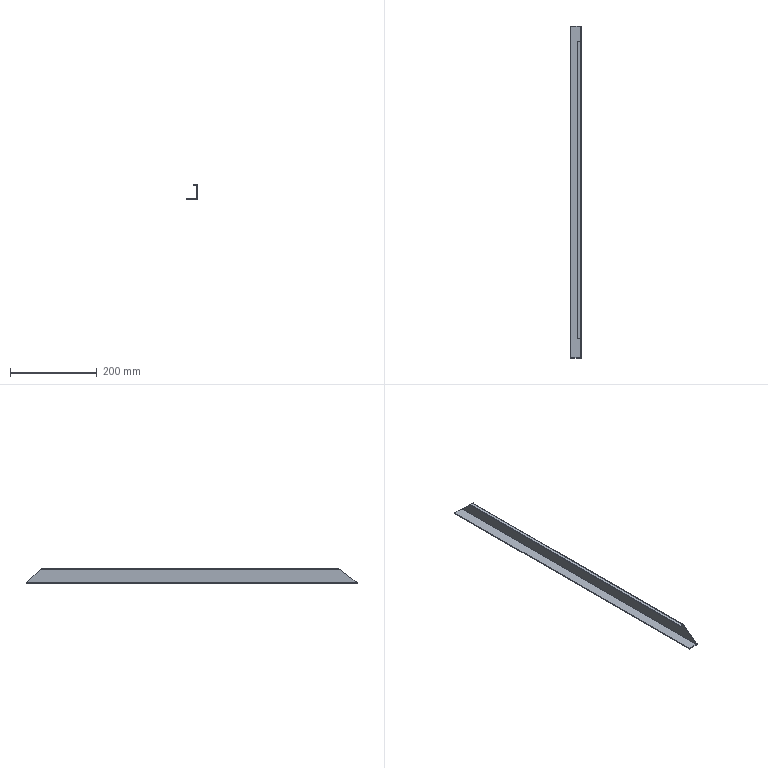Part | STEP file | Right Door Frame 1 | 1 solid | 28 faces | box 25 x 764 x 35 mm | volume 95446 mm3 | plane 22 | cylinder 6 | commonest cylinder face diameters 0.2 x2 0.4 x2 4.2 x2
STEP:
#1=CARTESIAN_POINT('',(-5.971,-678.242,30.9));
#2=VERTEX_POINT('',#1);
#3=CARTESIAN_POINT('',(-5.971,5.81,30.9));
#4=VERTEX_POINT('',#3);
#5=CARTESIAN_POINT('',(-5.971,0.,30.9));
#6=DIRECTION('',(0.,1.,0.));
#7=VECTOR('',#6,1000.);
#8=LINE('',#5,#7);
#9=EDGE_CURVE('',#2,#4,#8,.T.);
#10=ORIENTED_EDGE('',*,*,#9,.F.);
#11=CARTESIAN_POINT('',(-5.971,-678.242,33.));
#12=VERTEX_POINT('',#11);
#13=CARTESIAN_POINT('',(-5.971,-678.242,0.));
#14=DIRECTION('',(0.,0.,-1.));
#15=VECTOR('',#14,1000.);
#16=LINE('',#13,#15);
#17=EDGE_CURVE('',#12,#2,#16,.T.);
#18=ORIENTED_EDGE('',*,*,#17,.F.);
#19=CARTESIAN_POINT('',(-5.971,-721.39,0.2));
#20=VERTEX_POINT('',#19);
#21=CARTESIAN_POINT('',(-5.971,-721.39,0.2));
#22=DIRECTION('',(0.,0.7961,0.6052));
#23=VECTOR('',#22,1000.);
#24=LINE('',#21,#23);
#25=EDGE_CURVE('',#20,#12,#24,.T.);
#26=ORIENTED_EDGE('',*,*,#25,.F.);
#27=CARTESIAN_POINT('',(-5.971,-721.39,0.1));
#28=VERTEX_POINT('',#27);
#29=CARTESIAN_POINT('',(-5.971,-721.39,0.));
#30=DIRECTION('',(0.,0.,-1.));
#31=VECTOR('',#30,1000.);
#32=LINE('',#29,#31);
#33=EDGE_CURVE('',#20,#28,#32,.T.);
#34=ORIENTED_EDGE('',*,*,#33,.T.);
#35=CARTESIAN_POINT('',(-5.971,38.61,0.1));
#36=VERTEX_POINT('',#35);
#37=CARTESIAN_POINT('',(-5.971,0.,0.1));
#38=DIRECTION('',(0.,-1.,0.));
#39=VECTOR('',#38,1000.);
#40=LINE('',#37,#39);
#41=EDGE_CURVE('',#36,#28,#40,.T.);
#42=ORIENTED_EDGE('',*,*,#41,.F.);
#43=CARTESIAN_POINT('',(-5.971,38.61,0.2));
#44=VERTEX_POINT('',#43);
#45=CARTESIAN_POINT('',(-5.971,38.61,33.));
#46=DIRECTION('',(0.,0.,1.));
#47=VECTOR('',#46,1000.);
#48=LINE('',#45,#47);
#49=EDGE_CURVE('',#36,#44,#48,.T.);
#50=ORIENTED_EDGE('',*,*,#49,.T.);
#51=CARTESIAN_POINT('',(-5.971,5.81,33.));
#52=VERTEX_POINT('',#51);
#53=CARTESIAN_POINT('',(-5.971,5.81,33.));
#54=DIRECTION('',(0.,0.7071,-0.7071));
#55=VECTOR('',#54,1000.);
#56=LINE('',#53,#55);
#57=EDGE_CURVE('',#52,#44,#56,.T.);
#58=ORIENTED_EDGE('',*,*,#57,.F.);
#59=CARTESIAN_POINT('',(-5.971,5.81,0.));
#60=DIRECTION('',(0.,0.,1.));
#61=VECTOR('',#60,1000.);
#62=LINE('',#59,#61);
#63=EDGE_CURVE('',#4,#52,#62,.T.);
#64=ORIENTED_EDGE('',*,*,#63,.F.);
#65=EDGE_LOOP('',(#10,#18,#26,#34,#42,#50,#58,#64));
#66=FACE_OUTER_BOUND('',#65,.T.);
#67=CARTESIAN_POINT('',(-5.971,0.,0.));
#68=DIRECTION('',(-1.,0.,0.));
#69=DIRECTION('',(0.,0.,1.));
#70=AXIS2_PLACEMENT_3D('',#67,#68,#69);
#71=PLANE('',#70);
#72=ADVANCED_FACE('',(#66),#71,.F.);
#73=ORIENTED_EDGE('',*,*,#63,.T.);
#74=CARTESIAN_POINT('',(-7.971,5.81,33.));
#75=VERTEX_POINT('',#74);
#76=CARTESIAN_POINT('',(-7.971,5.81,33.));
#77=DIRECTION('',(-1.,0.,0.));
#78=VECTOR('',#77,1000.);
#79=LINE('',#76,#78);
#80=EDGE_CURVE('',#52,#75,#79,.T.);
#81=ORIENTED_EDGE('',*,*,#80,.T.);
#82=CARTESIAN_POINT('',(-7.971,5.81,32.998));
#83=VERTEX_POINT('',#82);
#84=CARTESIAN_POINT('',(-7.971,5.81,0.));
#85=DIRECTION('',(0.,0.,1.));
#86=VECTOR('',#85,1000.);
#87=LINE('',#84,#86);
#88=EDGE_CURVE('',#83,#75,#87,.T.);
#89=ORIENTED_EDGE('',*,*,#88,.F.);
#90=CARTESIAN_POINT('',(-8.071,5.81,30.9));
#91=DIRECTION('',(0.,1.,0.));
#92=DIRECTION('',(0.,0.,1.));
#93=AXIS2_PLACEMENT_3D('',#90,#91,#92);
#94=CIRCLE('',#93,2.1);
#95=EDGE_CURVE('',#83,#4,#94,.T.);
#96=ORIENTED_EDGE('',*,*,#95,.T.);
#97=EDGE_LOOP('',(#73,#81,#89,#96));
#98=FACE_OUTER_BOUND('',#97,.T.);
#99=CARTESIAN_POINT('',(-7.971,5.81,33.));
#100=DIRECTION('',(0.,-1.,0.));
#101=DIRECTION('',(0.,0.,-1.));
#102=AXIS2_PLACEMENT_3D('',#99,#100,#101);
#103=PLANE('',#102);
#104=ADVANCED_FACE('',(#98),#103,.T.);
#105=CARTESIAN_POINT('',(-7.971,-678.242,32.998));
#106=VERTEX_POINT('',#105);
#107=CARTESIAN_POINT('',(-8.071,-678.242,33.));
#108=VERTEX_POINT('',#107);
#109=CARTESIAN_POINT('',(-8.071,-678.242,30.9));
#110=DIRECTION('',(0.,-1.,0.));
#111=DIRECTION('',(0.,0.,-1.));
#112=AXIS2_PLACEMENT_3D('',#109,#110,#111);
#113=CIRCLE('',#112,2.1);
#114=EDGE_CURVE('',#106,#108,#113,.T.);
#115=ORIENTED_EDGE('',*,*,#114,.F.);
#116=CARTESIAN_POINT('',(-8.071,-678.242,30.9));
#117=DIRECTION('',(0.,1.,0.));
#118=DIRECTION('',(0.,0.,1.));
#119=AXIS2_PLACEMENT_3D('',#116,#117,#118);
#120=CIRCLE('',#119,2.1);
#121=EDGE_CURVE('',#106,#2,#120,.T.);
#122=ORIENTED_EDGE('',*,*,#121,.T.);
#123=ORIENTED_EDGE('',*,*,#9,.T.);
#124=ORIENTED_EDGE('',*,*,#95,.F.);
#125=CARTESIAN_POINT('',(-8.071,5.81,33.));
#126=VERTEX_POINT('',#125);
#127=CARTESIAN_POINT('',(-8.071,5.81,30.9));
#128=DIRECTION('',(0.,-1.,0.));
#129=DIRECTION('',(0.,0.,1.));
#130=AXIS2_PLACEMENT_3D('',#127,#128,#129);
#131=CIRCLE('',#130,2.1);
#132=EDGE_CURVE('',#83,#126,#131,.T.);
#133=ORIENTED_EDGE('',*,*,#132,.T.);
#134=CARTESIAN_POINT('',(-8.071,5.81,33.));
#135=DIRECTION('',(0.,-1.,0.));
#136=VECTOR('',#135,1000.);
#137=LINE('',#134,#136);
#138=EDGE_CURVE('',#126,#108,#137,.T.);
#139=ORIENTED_EDGE('',*,*,#138,.T.);
#140=EDGE_LOOP('',(#115,#122,#123,#124,#133,#139));
#141=FACE_OUTER_BOUND('',#140,.T.);
#142=CARTESIAN_POINT('',(-8.071,5.81,30.9));
#143=DIRECTION('',(0.,1.,0.));
#144=DIRECTION('',(0.,0.,1.));
#145=AXIS2_PLACEMENT_3D('',#142,#143,#144);
#146=CYLINDRICAL_SURFACE('',#145,2.1);
#147=ADVANCED_FACE('',(#141),#146,.T.);
#148=CARTESIAN_POINT('',(-7.971,-678.242,33.));
#149=VERTEX_POINT('',#148);
#150=CARTESIAN_POINT('',(-7.971,-678.242,0.));
#151=DIRECTION('',(0.,0.,-1.));
#152=VECTOR('',#151,1000.);
#153=LINE('',#150,#152);
#154=EDGE_CURVE('',#149,#106,#153,.T.);
#155=ORIENTED_EDGE('',*,*,#154,.F.);
#156=CARTESIAN_POINT('',(-7.971,-678.242,33.));
#157=DIRECTION('',(1.,0.,0.));
#158=VECTOR('',#157,1000.);
#159=LINE('',#156,#158);
#160=EDGE_CURVE('',#149,#12,#159,.T.);
#161=ORIENTED_EDGE('',*,*,#160,.T.);
#162=ORIENTED_EDGE('',*,*,#17,.T.);
#163=ORIENTED_EDGE('',*,*,#121,.F.);
#164=EDGE_LOOP('',(#155,#161,#162,#163));
#165=FACE_OUTER_BOUND('',#164,.T.);
#166=CARTESIAN_POINT('',(-7.971,-678.242,30.9));
#167=DIRECTION('',(0.,1.,0.));
#168=DIRECTION('',(0.,0.,1.));
#169=AXIS2_PLACEMENT_3D('',#166,#167,#168);
#170=PLANE('',#169);
#171=ADVANCED_FACE('',(#165),#170,.T.);
#172=CARTESIAN_POINT('',(-7.971,-721.39,0.2));
#173=VERTEX_POINT('',#172);
#174=CARTESIAN_POINT('',(-7.971,-721.39,0.2));
#175=DIRECTION('',(0.,0.7961,0.6052));
#176=VECTOR('',#175,1000.);
#177=LINE('',#174,#176);
#178=EDGE_CURVE('',#173,#149,#177,.T.);
#179=ORIENTED_EDGE('',*,*,#178,.F.);
#180=CARTESIAN_POINT('',(2.029,-721.39,0.2));
#181=DIRECTION('',(-1.,0.,0.));
#182=VECTOR('',#181,1000.);
#183=LINE('',#180,#182);
#184=EDGE_CURVE('',#20,#173,#183,.T.);
#185=ORIENTED_EDGE('',*,*,#184,.F.);
#186=ORIENTED_EDGE('',*,*,#25,.T.);
#187=ORIENTED_EDGE('',*,*,#160,.F.);
#188=EDGE_LOOP('',(#179,#185,#186,#187));
#189=FACE_OUTER_BOUND('',#188,.T.);
#190=CARTESIAN_POINT('',(2.029,-721.39,0.2));
#191=DIRECTION('',(0.,0.6052,-0.7961));
#192=DIRECTION('',(0.,0.7961,0.6052));
#193=AXIS2_PLACEMENT_3D('',#190,#191,#192);
#194=PLANE('',#193);
#195=ADVANCED_FACE('',(#189),#194,.F.);
#196=ORIENTED_EDGE('',*,*,#41,.T.);
#197=CARTESIAN_POINT('',(-8.071,-721.39,-2.));
#198=VERTEX_POINT('',#197);
#199=CARTESIAN_POINT('',(-8.071,-721.39,0.1));
#200=DIRECTION('',(0.,1.,0.));
#201=DIRECTION('',(0.,0.,1.));
#202=AXIS2_PLACEMENT_3D('',#199,#200,#201);
#203=CIRCLE('',#202,2.1);
#204=EDGE_CURVE('',#28,#198,#203,.T.);
#205=ORIENTED_EDGE('',*,*,#204,.T.);
#206=CARTESIAN_POINT('',(-8.071,38.61,-2.));
#207=VERTEX_POINT('',#206);
#208=CARTESIAN_POINT('',(-8.071,38.61,-2.));
#209=DIRECTION('',(0.,1.,0.));
#210=VECTOR('',#209,1000.);
#211=LINE('',#208,#210);
#212=EDGE_CURVE('',#198,#207,#211,.T.);
#213=ORIENTED_EDGE('',*,*,#212,.T.);
#214=CARTESIAN_POINT('',(-8.071,38.61,0.1));
#215=DIRECTION('',(0.,-1.,0.));
#216=DIRECTION('',(0.,0.,1.));
#217=AXIS2_PLACEMENT_3D('',#214,#215,#216);
#218=CIRCLE('',#217,2.1);
#219=EDGE_CURVE('',#207,#36,#218,.T.);
#220=ORIENTED_EDGE('',*,*,#219,.T.);
#221=EDGE_LOOP('',(#196,#205,#213,#220));
#222=FACE_OUTER_BOUND('',#221,.T.);
#223=CARTESIAN_POINT('',(-8.071,38.61,0.1));
#224=DIRECTION('',(0.,1.,0.));
#225=DIRECTION('',(0.,0.,1.));
#226=AXIS2_PLACEMENT_3D('',#223,#224,#225);
#227=CYLINDRICAL_SURFACE('',#226,2.1);
#228=ADVANCED_FACE('',(#222),#227,.T.);
#229=CARTESIAN_POINT('',(-7.971,38.61,0.2));
#230=VERTEX_POINT('',#229);
#231=CARTESIAN_POINT('',(-5.971,38.61,0.2));
#232=DIRECTION('',(1.,0.,0.));
#233=VECTOR('',#232,1000.);
#234=LINE('',#231,#233);
#235=EDGE_CURVE('',#230,#44,#234,.T.);
#236=ORIENTED_EDGE('',*,*,#235,.F.);
#237=CARTESIAN_POINT('',(-7.971,5.81,33.));
#238=DIRECTION('',(0.,0.7071,-0.7071));
#239=VECTOR('',#238,1000.);
#240=LINE('',#237,#239);
#241=EDGE_CURVE('',#75,#230,#240,.T.);
#242=ORIENTED_EDGE('',*,*,#241,.F.);
#243=ORIENTED_EDGE('',*,*,#80,.F.);
#244=ORIENTED_EDGE('',*,*,#57,.T.);
#245=EDGE_LOOP('',(#236,#242,#243,#244));
#246=FACE_OUTER_BOUND('',#245,.T.);
#247=CARTESIAN_POINT('',(-5.971,5.81,33.));
#248=DIRECTION('',(0.,-0.7071,-0.7071));
#249=DIRECTION('',(0.,0.7071,-0.7071));
#250=AXIS2_PLACEMENT_3D('',#247,#248,#249);
#251=PLANE('',#250);
#252=ADVANCED_FACE('',(#246),#251,.F.);
#253=CARTESIAN_POINT('',(-15.971,5.81,33.));
#254=VERTEX_POINT('',#253);
#255=CARTESIAN_POINT('',(0.,5.81,33.));
#256=DIRECTION('',(1.,0.,0.));
#257=VECTOR('',#256,1000.);
#258=LINE('',#255,#257);
#259=EDGE_CURVE('',#254,#126,#258,.T.);
#260=ORIENTED_EDGE('',*,*,#259,.F.);
#261=CARTESIAN_POINT('',(-15.971,-678.242,33.));
#262=VERTEX_POINT('',#261);
#263=CARTESIAN_POINT('',(-15.971,0.,33.));
#264=DIRECTION('',(0.,1.,0.));
#265=VECTOR('',#264,1000.);
#266=LINE('',#263,#265);
#267=EDGE_CURVE('',#262,#254,#266,.T.);
#268=ORIENTED_EDGE('',*,*,#267,.F.);
#269=CARTESIAN_POINT('',(0.,-678.242,33.));
#270=DIRECTION('',(-1.,0.,0.));
#271=VECTOR('',#270,1000.);
#272=LINE('',#269,#271);
#273=EDGE_CURVE('',#108,#262,#272,.T.);
#274=ORIENTED_EDGE('',*,*,#273,.F.);
#275=ORIENTED_EDGE('',*,*,#138,.F.);
#276=EDGE_LOOP('',(#260,#268,#274,#275));
#277=FACE_OUTER_BOUND('',#276,.T.);
#278=CARTESIAN_POINT('',(0.,0.,33.));
#279=DIRECTION('',(0.,0.,-1.));
#280=DIRECTION('',(-1.,0.,0.));
#281=AXIS2_PLACEMENT_3D('',#278,#279,#280);
#282=PLANE('',#281);
#283=ADVANCED_FACE('',(#277),#282,.F.);
#284=ORIENTED_EDGE('',*,*,#154,.T.);
#285=CARTESIAN_POINT('',(-7.971,-678.242,30.9));
#286=VERTEX_POINT('',#285);
#287=CARTESIAN_POINT('',(-7.971,-678.242,0.));
#288=DIRECTION('',(0.,0.,-1.));
#289=VECTOR('',#288,1000.);
#290=LINE('',#287,#289);
#291=EDGE_CURVE('',#106,#286,#290,.T.);
#292=ORIENTED_EDGE('',*,*,#291,.T.);
#293=CARTESIAN_POINT('',(-7.971,5.81,30.9));
#294=VERTEX_POINT('',#293);
#295=CARTESIAN_POINT('',(-7.971,0.,30.9));
#296=DIRECTION('',(0.,1.,0.));
#297=VECTOR('',#296,1000.);
#298=LINE('',#295,#297);
#299=EDGE_CURVE('',#286,#294,#298,.T.);
#300=ORIENTED_EDGE('',*,*,#299,.T.);
#301=CARTESIAN_POINT('',(-7.971,5.81,0.));
#302=DIRECTION('',(0.,0.,1.));
#303=VECTOR('',#302,1000.);
#304=LINE('',#301,#303);
#305=EDGE_CURVE('',#294,#83,#304,.T.);
#306=ORIENTED_EDGE('',*,*,#305,.T.);
#307=ORIENTED_EDGE('',*,*,#88,.T.);
#308=ORIENTED_EDGE('',*,*,#241,.T.);
#309=CARTESIAN_POINT('',(-7.971,38.61,0.1));
#310=VERTEX_POINT('',#309);
#311=CARTESIAN_POINT('',(-7.971,38.61,0.));
#312=DIRECTION('',(0.,0.,-1.));
#313=VECTOR('',#312,1000.);
#314=LINE('',#311,#313);
#315=EDGE_CURVE('',#230,#310,#314,.T.);
#316=ORIENTED_EDGE('',*,*,#315,.T.);
#317=CARTESIAN_POINT('',(-7.971,-721.39,0.1));
#318=VERTEX_POINT('',#317);
#319=CARTESIAN_POINT('',(-7.971,0.,0.1));
#320=DIRECTION('',(0.,-1.,0.));
#321=VECTOR('',#320,1000.);
#322=LINE('',#319,#321);
#323=EDGE_CURVE('',#310,#318,#322,.T.);
#324=ORIENTED_EDGE('',*,*,#323,.T.);
#325=CARTESIAN_POINT('',(-7.971,-721.39,0.));
#326=DIRECTION('',(0.,0.,1.));
#327=VECTOR('',#326,1000.);
#328=LINE('',#325,#327);
#329=EDGE_CURVE('',#318,#173,#328,.T.);
#330=ORIENTED_EDGE('',*,*,#329,.T.);
#331=ORIENTED_EDGE('',*,*,#178,.T.);
#332=EDGE_LOOP('',(#284,#292,#300,#306,#307,#308,#316,#324,#330,#331));
#333=FACE_OUTER_BOUND('',#332,.T.);
#334=CARTESIAN_POINT('',(-7.971,0.,0.));
#335=DIRECTION('',(-1.,0.,0.));
#336=DIRECTION('',(0.,0.,1.));
#337=AXIS2_PLACEMENT_3D('',#334,#335,#336);
#338=PLANE('',#337);
#339=ADVANCED_FACE('',(#333),#338,.T.);
#340=ORIENTED_EDGE('',*,*,#184,.T.);
#341=ORIENTED_EDGE('',*,*,#329,.F.);
#342=CARTESIAN_POINT('',(-8.071,-721.39,0.));
#343=VERTEX_POINT('',#342);
#344=CARTESIAN_POINT('',(-8.071,-721.39,0.1));
#345=DIRECTION('',(0.,1.,0.));
#346=DIRECTION('',(0.,0.,1.));
#347=AXIS2_PLACEMENT_3D('',#344,#345,#346);
#348=CIRCLE('',#347,0.1);
#349=EDGE_CURVE('',#318,#343,#348,.T.);
#350=ORIENTED_EDGE('',*,*,#349,.T.);
#351=CARTESIAN_POINT('',(-8.471,-721.39,0.));
#352=VERTEX_POINT('',#351);
#353=CARTESIAN_POINT('',(-8.071,-721.39,0.));
#354=DIRECTION('',(-1.,0.,0.));
#355=VECTOR('',#354,1000.);
#356=LINE('',#353,#355);
#357=EDGE_CURVE('',#343,#352,#356,.T.);
#358=ORIENTED_EDGE('',*,*,#357,.T.);
#359=CARTESIAN_POINT('',(-8.471,-721.39,-2.));
#360=VERTEX_POINT('',#359);
#361=CARTESIAN_POINT('',(-8.471,-721.39,0.));
#362=DIRECTION('',(0.,0.,-1.));
#363=VECTOR('',#362,1000.);
#364=LINE('',#361,#363);
#365=EDGE_CURVE('',#352,#360,#364,.T.);
#366=ORIENTED_EDGE('',*,*,#365,.T.);
#367=CARTESIAN_POINT('',(0.,-721.39,-2.));
#368=DIRECTION('',(1.,0.,0.));
#369=VECTOR('',#368,1000.);
#370=LINE('',#367,#369);
#371=EDGE_CURVE('',#360,#198,#370,.T.);
#372=ORIENTED_EDGE('',*,*,#371,.T.);
#373=ORIENTED_EDGE('',*,*,#204,.F.);
#374=ORIENTED_EDGE('',*,*,#33,.F.);
#375=EDGE_LOOP('',(#340,#341,#350,#358,#366,#372,#373,#374));
#376=FACE_OUTER_BOUND('',#375,.T.);
#377=CARTESIAN_POINT('',(-5.971,-721.39,0.));
#378=DIRECTION('',(0.,1.,0.));
#379=DIRECTION('',(-1.,0.,0.));
#380=AXIS2_PLACEMENT_3D('',#377,#378,#379);
#381=PLANE('',#380);
#382=ADVANCED_FACE('',(#376),#381,.F.);
#383=CARTESIAN_POINT('',(-8.071,38.61,0.));
#384=VERTEX_POINT('',#383);
#385=CARTESIAN_POINT('',(-8.071,38.61,0.1));
#386=DIRECTION('',(0.,1.,0.));
#387=DIRECTION('',(0.,0.,1.));
#388=AXIS2_PLACEMENT_3D('',#385,#386,#387);
#389=CIRCLE('',#388,0.1);
#390=EDGE_CURVE('',#310,#384,#389,.T.);
#391=ORIENTED_EDGE('',*,*,#390,.F.);
#392=ORIENTED_EDGE('',*,*,#315,.F.);
#393=ORIENTED_EDGE('',*,*,#235,.T.);
#394=ORIENTED_EDGE('',*,*,#49,.F.);
#395=ORIENTED_EDGE('',*,*,#219,.F.);
#396=CARTESIAN_POINT('',(-8.471,38.61,-2.));
#397=VERTEX_POINT('',#396);
#398=CARTESIAN_POINT('',(0.,38.61,-2.));
#399=DIRECTION('',(-1.,0.,0.));
#400=VECTOR('',#399,1000.);
#401=LINE('',#398,#400);
#402=EDGE_CURVE('',#207,#397,#401,.T.);
#403=ORIENTED_EDGE('',*,*,#402,.T.);
#404=CARTESIAN_POINT('',(-8.471,38.61,0.));
#405=VERTEX_POINT('',#404);
#406=CARTESIAN_POINT('',(-8.471,38.61,0.));
#407=DIRECTION('',(0.,0.,1.));
#408=VECTOR('',#407,1000.);
#409=LINE('',#406,#408);
#410=EDGE_CURVE('',#397,#405,#409,.T.);
#411=ORIENTED_EDGE('',*,*,#410,.T.);
#412=CARTESIAN_POINT('',(-8.471,38.61,0.));
#413=DIRECTION('',(1.,0.,0.));
#414=VECTOR('',#413,1000.);
#415=LINE('',#412,#414);
#416=EDGE_CURVE('',#405,#384,#415,.T.);
#417=ORIENTED_EDGE('',*,*,#416,.T.);
#418=EDGE_LOOP('',(#391,#392,#393,#394,#395,#403,#411,#417));
#419=FACE_OUTER_BOUND('',#418,.T.);
#420=CARTESIAN_POINT('',(-8.071,38.61,0.1));
#421=DIRECTION('',(0.,-1.,0.));
#422=DIRECTION('',(0.,0.,-1.));
#423=AXIS2_PLACEMENT_3D('',#420,#421,#422);
#424=PLANE('',#423);
#425=ADVANCED_FACE('',(#419),#424,.F.);
#426=CARTESIAN_POINT('',(-8.471,39.01,-2.));
#427=VERTEX_POINT('',#426);
#428=CARTESIAN_POINT('',(-8.471,38.81,-2.));
#429=DIRECTION('',(0.,0.,1.));
#430=DIRECTION('',(0.,1.,0.));
#431=AXIS2_PLACEMENT_3D('',#428,#429,#430);
#432=CIRCLE('',#431,0.2);
#433=EDGE_CURVE('',#427,#397,#432,.T.);
#434=ORIENTED_EDGE('',*,*,#433,.T.);
#435=ORIENTED_EDGE('',*,*,#402,.F.);
#436=ORIENTED_EDGE('',*,*,#212,.F.);
#437=ORIENTED_EDGE('',*,*,#371,.F.);
#438=CARTESIAN_POINT('',(-8.471,-721.79,-2.));
#439=VERTEX_POINT('',#438);
#440=CARTESIAN_POINT('',(-8.471,-721.59,-2.));
#441=DIRECTION('',(0.,0.,1.));
#442=DIRECTION('',(0.,1.,0.));
#443=AXIS2_PLACEMENT_3D('',#440,#441,#442);
#444=CIRCLE('',#443,0.2);
#445=EDGE_CURVE('',#360,#439,#444,.T.);
#446=ORIENTED_EDGE('',*,*,#445,.T.);
#447=CARTESIAN_POINT('',(-5.971,-721.79,-2.));
#448=VERTEX_POINT('',#447);
#449=CARTESIAN_POINT('',(0.,-721.79,-2.));
#450=DIRECTION('',(-1.,0.,0.));
#451=VECTOR('',#450,1000.);
#452=LINE('',#449,#451);
#453=EDGE_CURVE('',#448,#439,#452,.T.);
#454=ORIENTED_EDGE('',*,*,#453,.F.);
#455=CARTESIAN_POINT('',(-5.971,-723.39,-2.));
#456=VERTEX_POINT('',#455);
#457=CARTESIAN_POINT('',(-5.971,40.61,-2.));
#458=DIRECTION('',(0.,1.,0.));
#459=VECTOR('',#458,1000.);
#460=LINE('',#457,#459);
#461=EDGE_CURVE('',#456,#448,#460,.T.);
#462=ORIENTED_EDGE('',*,*,#461,.F.);
#463=CARTESIAN_POINT('',(-30.971,-723.39,-2.));
#464=VERTEX_POINT('',#463);
#465=CARTESIAN_POINT('',(0.,-723.39,-2.));
#466=DIRECTION('',(1.,0.,0.));
#467=VECTOR('',#466,1000.);
#468=LINE('',#465,#467);
#469=EDGE_CURVE('',#464,#456,#468,.T.);
#470=ORIENTED_EDGE('',*,*,#469,.F.);
#471=CARTESIAN_POINT('',(-30.971,40.61,-2.));
#472=VERTEX_POINT('',#471);
#473=CARTESIAN_POINT('',(-30.971,0.,-2.));
#474=DIRECTION('',(0.,-1.,0.));
#475=VECTOR('',#474,1000.);
#476=LINE('',#473,#475);
#477=EDGE_CURVE('',#472,#464,#476,.T.);
#478=ORIENTED_EDGE('',*,*,#477,.F.);
#479=CARTESIAN_POINT('',(-5.971,40.61,-2.));
#480=VERTEX_POINT('',#479);
#481=CARTESIAN_POINT('',(0.,40.61,-2.));
#482=DIRECTION('',(-1.,0.,0.));
#483=VECTOR('',#482,1000.);
#484=LINE('',#481,#483);
#485=EDGE_CURVE('',#480,#472,#484,.T.);
#486=ORIENTED_EDGE('',*,*,#485,.F.);
#487=CARTESIAN_POINT('',(-5.971,39.01,-2.));
#488=VERTEX_POINT('',#487);
#489=CARTESIAN_POINT('',(-5.971,40.61,-2.));
#490=DIRECTION('',(0.,1.,0.));
#491=VECTOR('',#490,1000.);
#492=LINE('',#489,#491);
#493=EDGE_CURVE('',#488,#480,#492,.T.);
#494=ORIENTED_EDGE('',*,*,#493,.F.);
#495=CARTESIAN_POINT('',(0.,39.01,-2.));
#496=DIRECTION('',(1.,0.,0.));
#497=VECTOR('',#496,1000.);
#498=LINE('',#495,#497);
#499=EDGE_CURVE('',#427,#488,#498,.T.);
#500=ORIENTED_EDGE('',*,*,#499,.F.);
#501=EDGE_LOOP('',(#434,#435,#436,#437,#446,#454,#462,#470,#478,#486,#494,#500));
#502=FACE_OUTER_BOUND('',#501,.T.);
#503=CARTESIAN_POINT('',(0.,0.,-2.));
#504=DIRECTION('',(0.,0.,1.));
#505=DIRECTION('',(1.,0.,0.));
#506=AXIS2_PLACEMENT_3D('',#503,#504,#505);
#507=PLANE('',#506);
#508=ADVANCED_FACE('',(#502),#507,.F.);
#509=CARTESIAN_POINT('',(-15.971,5.81,31.));
#510=VERTEX_POINT('',#509);
#511=CARTESIAN_POINT('',(-8.071,5.81,31.));
#512=VERTEX_POINT('',#511);
#513=CARTESIAN_POINT('',(-15.971,5.81,31.));
#514=DIRECTION('',(1.,0.,0.));
#515=VECTOR('',#514,1000.);
#516=LINE('',#513,#515);
#517=EDGE_CURVE('',#510,#512,#516,.T.);
#518=ORIENTED_EDGE('',*,*,#517,.F.);
#519=CARTESIAN_POINT('',(-15.971,5.81,33.));
#520=DIRECTION('',(0.,0.,-1.));
#521=VECTOR('',#520,1000.);
#522=LINE('',#519,#521);
#523=EDGE_CURVE('',#254,#510,#522,.T.);
#524=ORIENTED_EDGE('',*,*,#523,.F.);
#525=ORIENTED_EDGE('',*,*,#259,.T.);
#526=ORIENTED_EDGE('',*,*,#132,.F.);
#527=ORIENTED_EDGE('',*,*,#305,.F.);
#528=CARTESIAN_POINT('',(-8.071,5.81,30.9));
#529=DIRECTION('',(0.,1.,0.));
#530=DIRECTION('',(0.,0.,1.));
#531=AXIS2_PLACEMENT_3D('',#528,#529,#530);
#532=CIRCLE('',#531,0.1);
#533=EDGE_CURVE('',#512,#294,#532,.T.);
#534=ORIENTED_EDGE('',*,*,#533,.F.);
#535=EDGE_LOOP('',(#518,#524,#525,#526,#527,#534));
#536=FACE_OUTER_BOUND('',#535,.T.);
#537=CARTESIAN_POINT('',(-15.971,5.81,33.));
#538=DIRECTION('',(0.,-1.,0.));
#539=DIRECTION('',(1.,0.,0.));
#540=AXIS2_PLACEMENT_3D('',#537,#538,#539);
#541=PLANE('',#540);
#542=ADVANCED_FACE('',(#536),#541,.F.);
#543=CARTESIAN_POINT('',(-15.971,-678.242,31.));
#544=VERTEX_POINT('',#543);
#545=CARTESIAN_POINT('',(-15.971,-678.242,33.));
#546=DIRECTION('',(0.,0.,-1.));
#547=VECTOR('',#546,1000.);
#548=LINE('',#545,#547);
#549=EDGE_CURVE('',#262,#544,#548,.T.);
#550=ORIENTED_EDGE('',*,*,#549,.F.);
#551=ORIENTED_EDGE('',*,*,#267,.T.);
#552=ORIENTED_EDGE('',*,*,#523,.T.);
#553=CARTESIAN_POINT('',(-15.971,-678.242,31.));
#554=DIRECTION('',(0.,1.,0.));
#555=VECTOR('',#554,1000.);
#556=LINE('',#553,#555);
#557=EDGE_CURVE('',#544,#510,#556,.T.);
#558=ORIENTED_EDGE('',*,*,#557,.F.);
#559=EDGE_LOOP('',(#550,#551,#552,#558));
#560=FACE_OUTER_BOUND('',#559,.T.);
#561=CARTESIAN_POINT('',(-15.971,-678.242,33.));
#562=DIRECTION('',(1.,0.,0.));
#563=DIRECTION('',(0.,0.,-1.));
#564=AXIS2_PLACEMENT_3D('',#561,#562,#563);
#565=PLANE('',#564);
#566=ADVANCED_FACE('',(#560),#565,.F.);
#567=ORIENTED_EDGE('',*,*,#273,.T.);
#568=ORIENTED_EDGE('',*,*,#549,.T.);
#569=CARTESIAN_POINT('',(-8.071,-678.242,31.));
#570=VERTEX_POINT('',#569);
#571=CARTESIAN_POINT('',(-7.971,-678.242,31.));
#572=DIRECTION('',(-1.,0.,0.));
#573=VECTOR('',#572,1000.);
#574=LINE('',#571,#573);
#575=EDGE_CURVE('',#570,#544,#574,.T.);
#576=ORIENTED_EDGE('',*,*,#575,.F.);
#577=CARTESIAN_POINT('',(-8.071,-678.242,30.9));
#578=DIRECTION('',(0.,1.,0.));
#579=DIRECTION('',(0.,0.,1.));
#580=AXIS2_PLACEMENT_3D('',#577,#578,#579);
#581=CIRCLE('',#580,0.1);
#582=EDGE_CURVE('',#570,#286,#581,.T.);
#583=ORIENTED_EDGE('',*,*,#582,.T.);
#584=ORIENTED_EDGE('',*,*,#291,.F.);
#585=ORIENTED_EDGE('',*,*,#114,.T.);
#586=EDGE_LOOP('',(#567,#568,#576,#583,#584,#585));
#587=FACE_OUTER_BOUND('',#586,.T.);
#588=CARTESIAN_POINT('',(-7.971,-678.242,33.));
#589=DIRECTION('',(0.,1.,0.));
#590=DIRECTION('',(0.,0.,1.));
#591=AXIS2_PLACEMENT_3D('',#588,#589,#590);
#592=PLANE('',#591);
#593=ADVANCED_FACE('',(#587),#592,.F.);
#594=ORIENTED_EDGE('',*,*,#349,.F.);
#595=ORIENTED_EDGE('',*,*,#323,.F.);
#596=ORIENTED_EDGE('',*,*,#390,.T.);
#597=CARTESIAN_POINT('',(-8.071,38.61,0.));
#598=DIRECTION('',(0.,1.,0.));
#599=VECTOR('',#598,1000.);
#600=LINE('',#597,#599);
#601=EDGE_CURVE('',#343,#384,#600,.T.);
#602=ORIENTED_EDGE('',*,*,#601,.F.);
#603=EDGE_LOOP('',(#594,#595,#596,#602));
#604=FACE_OUTER_BOUND('',#603,.T.);
#605=CARTESIAN_POINT('',(-8.071,38.61,0.1));
#606=DIRECTION('',(0.,1.,0.));
#607=DIRECTION('',(0.,0.,1.));
#608=AXIS2_PLACEMENT_3D('',#605,#606,#607);
#609=CYLINDRICAL_SURFACE('',#608,0.1);
#610=ADVANCED_FACE('',(#604),#609,.F.);
#611=ORIENTED_EDGE('',*,*,#582,.F.);
#612=CARTESIAN_POINT('',(-8.071,5.81,31.));
#613=DIRECTION('',(0.,-1.,0.));
#614=VECTOR('',#613,1000.);
#615=LINE('',#612,#614);
#616=EDGE_CURVE('',#512,#570,#615,.T.);
#617=ORIENTED_EDGE('',*,*,#616,.F.);
#618=ORIENTED_EDGE('',*,*,#533,.T.);
#619=ORIENTED_EDGE('',*,*,#299,.F.);
#620=EDGE_LOOP('',(#611,#617,#618,#619));
#621=FACE_OUTER_BOUND('',#620,.T.);
#622=CARTESIAN_POINT('',(-8.071,5.81,30.9));
#623=DIRECTION('',(0.,1.,0.));
#624=DIRECTION('',(0.,0.,1.));
#625=AXIS2_PLACEMENT_3D('',#622,#623,#624);
#626=CYLINDRICAL_SURFACE('',#625,0.1);
#627=ADVANCED_FACE('',(#621),#626,.F.);
#628=CARTESIAN_POINT('',(-5.971,39.01,0.));
#629=VERTEX_POINT('',#628);
#630=CARTESIAN_POINT('',(-5.971,39.01,0.));
#631=DIRECTION('',(0.,0.,1.));
#632=VECTOR('',#631,1000.);
#633=LINE('',#630,#632);
#634=EDGE_CURVE('',#488,#629,#633,.T.);
#635=ORIENTED_EDGE('',*,*,#634,.T.);
#636=CARTESIAN_POINT('',(-8.471,39.01,0.));
#637=VERTEX_POINT('',#636);
#638=CARTESIAN_POINT('',(-5.971,39.01,0.));
#639=DIRECTION('',(-1.,0.,0.));
#640=VECTOR('',#639,1000.);
#641=LINE('',#638,#640);
#642=EDGE_CURVE('',#629,#637,#641,.T.);
#643=ORIENTED_EDGE('',*,*,#642,.T.);
#644=CARTESIAN_POINT('',(-8.471,39.01,0.));
#645=DIRECTION('',(0.,0.,-1.));
#646=VECTOR('',#645,1000.);
#647=LINE('',#644,#646);
#648=EDGE_CURVE('',#637,#427,#647,.T.);
#649=ORIENTED_EDGE('',*,*,#648,.T.);
#650=ORIENTED_EDGE('',*,*,#499,.T.);
#651=EDGE_LOOP('',(#635,#643,#649,#650));
#652=FACE_OUTER_BOUND('',#651,.T.);
#653=CARTESIAN_POINT('',(-5.971,39.01,0.));
#654=DIRECTION('',(0.,-1.,0.));
#655=DIRECTION('',(0.,0.,-1.));
#656=AXIS2_PLACEMENT_3D('',#653,#654,#655);
#657=PLANE('',#656);
#658=ADVANCED_FACE('',(#652),#657,.T.);
#659=CARTESIAN_POINT('',(-8.471,-721.79,0.));
#660=VERTEX_POINT('',#659);
#661=CARTESIAN_POINT('',(-8.471,-721.79,0.));
#662=DIRECTION('',(0.,0.,1.));
#663=VECTOR('',#662,1000.);
#664=LINE('',#661,#663);
#665=EDGE_CURVE('',#439,#660,#664,.T.);
#666=ORIENTED_EDGE('',*,*,#665,.T.);
#667=CARTESIAN_POINT('',(-5.971,-721.79,0.));
#668=VERTEX_POINT('',#667);
#669=CARTESIAN_POINT('',(-8.471,-721.79,0.));
#670=DIRECTION('',(1.,0.,0.));
#671=VECTOR('',#670,1000.);
#672=LINE('',#669,#671);
#673=EDGE_CURVE('',#660,#668,#672,.T.);
#674=ORIENTED_EDGE('',*,*,#673,.T.);
#675=CARTESIAN_POINT('',(-5.971,-721.79,0.));
#676=DIRECTION('',(0.,0.,-1.));
#677=VECTOR('',#676,1000.);
#678=LINE('',#675,#677);
#679=EDGE_CURVE('',#668,#448,#678,.T.);
#680=ORIENTED_EDGE('',*,*,#679,.T.);
#681=ORIENTED_EDGE('',*,*,#453,.T.);
#682=EDGE_LOOP('',(#666,#674,#680,#681));
#683=FACE_OUTER_BOUND('',#682,.T.);
#684=CARTESIAN_POINT('',(-8.471,-721.79,0.));
#685=DIRECTION('',(0.,1.,0.));
#686=DIRECTION('',(0.,0.,1.));
#687=AXIS2_PLACEMENT_3D('',#684,#685,#686);
#688=PLANE('',#687);
#689=ADVANCED_FACE('',(#683),#688,.T.);
#690=ORIENTED_EDGE('',*,*,#469,.T.);
#691=CARTESIAN_POINT('',(-5.971,-723.39,0.));
#692=VERTEX_POINT('',#691);
#693=CARTESIAN_POINT('',(-5.971,-723.39,-2.));
#694=DIRECTION('',(0.,0.,1.));
#695=VECTOR('',#694,1000.);
#696=LINE('',#693,#695);
#697=EDGE_CURVE('',#456,#692,#696,.T.);
#698=ORIENTED_EDGE('',*,*,#697,.T.);
#699=CARTESIAN_POINT('',(-30.971,-723.39,0.));
#700=VERTEX_POINT('',#699);
#701=CARTESIAN_POINT('',(-30.971,-723.39,0.));
#702=DIRECTION('',(-1.,0.,0.));
#703=VECTOR('',#702,1000.);
#704=LINE('',#701,#703);
#705=EDGE_CURVE('',#692,#700,#704,.T.);
#706=ORIENTED_EDGE('',*,*,#705,.T.);
#707=CARTESIAN_POINT('',(-30.971,-723.39,-2.));
#708=DIRECTION('',(0.,0.,-1.));
#709=VECTOR('',#708,1000.);
#710=LINE('',#707,#709);
#711=EDGE_CURVE('',#700,#464,#710,.T.);
#712=ORIENTED_EDGE('',*,*,#711,.T.);
#713=EDGE_LOOP('',(#690,#698,#706,#712));
#714=FACE_OUTER_BOUND('',#713,.T.);
#715=CARTESIAN_POINT('',(-30.971,-723.39,-2.));
#716=DIRECTION('',(0.,-1.,0.));
#717=DIRECTION('',(0.,0.,-1.));
#718=AXIS2_PLACEMENT_3D('',#715,#716,#717);
#719=PLANE('',#718);
#720=ADVANCED_FACE('',(#714),#719,.T.);
#721=ORIENTED_EDGE('',*,*,#477,.T.);
#722=ORIENTED_EDGE('',*,*,#711,.F.);
#723=CARTESIAN_POINT('',(-30.971,40.61,0.));
#724=VERTEX_POINT('',#723);
#725=CARTESIAN_POINT('',(-30.971,40.61,0.));
#726=DIRECTION('',(0.,1.,0.));
#727=VECTOR('',#726,1000.);
#728=LINE('',#725,#727);
#729=EDGE_CURVE('',#700,#724,#728,.T.);
#730=ORIENTED_EDGE('',*,*,#729,.T.);
#731=CARTESIAN_POINT('',(-30.971,40.61,-2.));
#732=DIRECTION('',(0.,0.,-1.));
#733=VECTOR('',#732,1000.);
#734=LINE('',#731,#733);
#735=EDGE_CURVE('',#724,#472,#734,.T.);
#736=ORIENTED_EDGE('',*,*,#735,.T.);
#737=EDGE_LOOP('',(#721,#722,#730,#736));
#738=FACE_OUTER_BOUND('',#737,.T.);
#739=CARTESIAN_POINT('',(-30.971,40.61,-2.));
#740=DIRECTION('',(-1.,0.,0.));
#741=DIRECTION('',(0.,-1.,0.));
#742=AXIS2_PLACEMENT_3D('',#739,#740,#741);
#743=PLANE('',#742);
#744=ADVANCED_FACE('',(#738),#743,.T.);
#745=ORIENTED_EDGE('',*,*,#485,.T.);
#746=ORIENTED_EDGE('',*,*,#735,.F.);
#747=CARTESIAN_POINT('',(-5.971,40.61,0.));
#748=VERTEX_POINT('',#747);
#749=CARTESIAN_POINT('',(-30.971,40.61,0.));
#750=DIRECTION('',(1.,0.,0.));
#751=VECTOR('',#750,1000.);
#752=LINE('',#749,#751);
#753=EDGE_CURVE('',#724,#748,#752,.T.);
#754=ORIENTED_EDGE('',*,*,#753,.T.);
#755=CARTESIAN_POINT('',(-5.971,40.61,-2.));
#756=DIRECTION('',(0.,0.,-1.));
#757=VECTOR('',#756,1000.);
#758=LINE('',#755,#757);
#759=EDGE_CURVE('',#748,#480,#758,.T.);
#760=ORIENTED_EDGE('',*,*,#759,.T.);
#761=EDGE_LOOP('',(#745,#746,#754,#760));
#762=FACE_OUTER_BOUND('',#761,.T.);
#763=CARTESIAN_POINT('',(-30.971,40.61,-2.));
#764=DIRECTION('',(0.,1.,0.));
#765=DIRECTION('',(0.,0.,1.));
#766=AXIS2_PLACEMENT_3D('',#763,#764,#765);
#767=PLANE('',#766);
#768=ADVANCED_FACE('',(#762),#767,.T.);
#769=ORIENTED_EDGE('',*,*,#575,.T.);
#770=ORIENTED_EDGE('',*,*,#557,.T.);
#771=ORIENTED_EDGE('',*,*,#517,.T.);
#772=ORIENTED_EDGE('',*,*,#616,.T.);
#773=EDGE_LOOP('',(#769,#770,#771,#772));
#774=FACE_OUTER_BOUND('',#773,.T.);
#775=CARTESIAN_POINT('',(0.,0.,31.));
#776=DIRECTION('',(0.,0.,-1.));
#777=DIRECTION('',(-1.,0.,0.));
#778=AXIS2_PLACEMENT_3D('',#775,#776,#777);
#779=PLANE('',#778);
#780=ADVANCED_FACE('',(#774),#779,.T.);
#781=ORIENTED_EDGE('',*,*,#601,.T.);
#782=ORIENTED_EDGE('',*,*,#416,.F.);
#783=CARTESIAN_POINT('',(-8.471,38.81,0.));
#784=DIRECTION('',(0.,0.,-1.));
#785=DIRECTION('',(0.,1.,0.));
#786=AXIS2_PLACEMENT_3D('',#783,#784,#785);
#787=CIRCLE('',#786,0.2);
#788=EDGE_CURVE('',#405,#637,#787,.T.);
#789=ORIENTED_EDGE('',*,*,#788,.T.);
#790=ORIENTED_EDGE('',*,*,#642,.F.);
#791=CARTESIAN_POINT('',(-5.971,0.,0.));
#792=DIRECTION('',(0.,1.,0.));
#793=VECTOR('',#792,1000.);
#794=LINE('',#791,#793);
#795=EDGE_CURVE('',#629,#748,#794,.T.);
#796=ORIENTED_EDGE('',*,*,#795,.T.);
#797=ORIENTED_EDGE('',*,*,#753,.F.);
#798=ORIENTED_EDGE('',*,*,#729,.F.);
#799=ORIENTED_EDGE('',*,*,#705,.F.);
#800=CARTESIAN_POINT('',(-5.971,0.,0.));
#801=DIRECTION('',(0.,1.,0.));
#802=VECTOR('',#801,1000.);
#803=LINE('',#800,#802);
#804=EDGE_CURVE('',#692,#668,#803,.T.);
#805=ORIENTED_EDGE('',*,*,#804,.T.);
#806=ORIENTED_EDGE('',*,*,#673,.F.);
#807=CARTESIAN_POINT('',(-8.471,-721.59,0.));
#808=DIRECTION('',(0.,0.,-1.));
#809=DIRECTION('',(0.,1.,0.));
#810=AXIS2_PLACEMENT_3D('',#807,#808,#809);
#811=CIRCLE('',#810,0.2);
#812=EDGE_CURVE('',#660,#352,#811,.T.);
#813=ORIENTED_EDGE('',*,*,#812,.T.);
#814=ORIENTED_EDGE('',*,*,#357,.F.);
#815=EDGE_LOOP('',(#781,#782,#789,#790,#796,#797,#798,#799,#805,#806,#813,#814));
#816=FACE_OUTER_BOUND('',#815,.T.);
#817=CARTESIAN_POINT('',(0.,0.,0.));
#818=DIRECTION('',(0.,0.,1.));
#819=DIRECTION('',(1.,0.,0.));
#820=AXIS2_PLACEMENT_3D('',#817,#818,#819);
#821=PLANE('',#820);
#822=ADVANCED_FACE('',(#816),#821,.T.);
#823=ORIENTED_EDGE('',*,*,#445,.F.);
#824=ORIENTED_EDGE('',*,*,#365,.F.);
#825=ORIENTED_EDGE('',*,*,#812,.F.);
#826=ORIENTED_EDGE('',*,*,#665,.F.);
#827=EDGE_LOOP('',(#823,#824,#825,#826));
#828=FACE_OUTER_BOUND('',#827,.T.);
#829=CARTESIAN_POINT('',(-8.471,-721.59,0.));
#830=DIRECTION('',(0.,0.,-1.));
#831=DIRECTION('',(0.,1.,0.));
#832=AXIS2_PLACEMENT_3D('',#829,#830,#831);
#833=CYLINDRICAL_SURFACE('',#832,0.2);
#834=ADVANCED_FACE('',(#828),#833,.F.);
#835=ORIENTED_EDGE('',*,*,#433,.F.);
#836=ORIENTED_EDGE('',*,*,#648,.F.);
#837=ORIENTED_EDGE('',*,*,#788,.F.);
#838=ORIENTED_EDGE('',*,*,#410,.F.);
#839=EDGE_LOOP('',(#835,#836,#837,#838));
#840=FACE_OUTER_BOUND('',#839,.T.);
#841=CARTESIAN_POINT('',(-8.471,38.81,0.));
#842=DIRECTION('',(0.,0.,-1.));
#843=DIRECTION('',(0.,1.,0.));
#844=AXIS2_PLACEMENT_3D('',#841,#842,#843);
#845=CYLINDRICAL_SURFACE('',#844,0.2);
#846=ADVANCED_FACE('',(#840),#845,.F.);
#847=ORIENTED_EDGE('',*,*,#493,.T.);
#848=ORIENTED_EDGE('',*,*,#759,.F.);
#849=ORIENTED_EDGE('',*,*,#795,.F.);
#850=ORIENTED_EDGE('',*,*,#634,.F.);
#851=EDGE_LOOP('',(#847,#848,#849,#850));
#852=FACE_OUTER_BOUND('',#851,.T.);
#853=CARTESIAN_POINT('',(-5.971,40.61,-2.));
#854=DIRECTION('',(1.,0.,0.));
#855=DIRECTION('',(0.,1.,0.));
#856=AXIS2_PLACEMENT_3D('',#853,#854,#855);
#857=PLANE('',#856);
#858=ADVANCED_FACE('',(#852),#857,.T.);
#859=ORIENTED_EDGE('',*,*,#804,.F.);
#860=ORIENTED_EDGE('',*,*,#697,.F.);
#861=ORIENTED_EDGE('',*,*,#461,.T.);
#862=ORIENTED_EDGE('',*,*,#679,.F.);
#863=EDGE_LOOP('',(#859,#860,#861,#862));
#864=FACE_OUTER_BOUND('',#863,.T.);
#865=CARTESIAN_POINT('',(-5.971,40.61,-2.));
#866=DIRECTION('',(1.,0.,0.));
#867=DIRECTION('',(0.,1.,0.));
#868=AXIS2_PLACEMENT_3D('',#865,#866,#867);
#869=PLANE('',#868);
#870=ADVANCED_FACE('',(#864),#869,.T.);
#871=CLOSED_SHELL('',(#72,#104,#147,#171,#195,#228,#252,#283,#339,#382,#425,#508,#542,#566,#593,#610,#627,#658,#689,#720,#744,#768,#780,#822,#834,#846,#858,#870));
#872=MANIFOLD_SOLID_BREP('',#871);
#873=CARTESIAN_POINT('',(0.,0.,0.));
#874=DIRECTION('',(0.,0.,1.));
#875=DIRECTION('',(1.,0.,0.));
#876=AXIS2_PLACEMENT_3D('',#873,#874,#875);
#877=(LENGTH_UNIT()NAMED_UNIT(*)SI_UNIT(.MILLI.,.METRE.));
#878=UNCERTAINTY_MEASURE_WITH_UNIT(LENGTH_MEASURE(0.00001),#877,'','');
#879=(NAMED_UNIT(*)PLANE_ANGLE_UNIT()SI_UNIT($,.RADIAN.));
#880=(NAMED_UNIT(*)SI_UNIT($,.STERADIAN.)SOLID_ANGLE_UNIT());
#881=(GEOMETRIC_REPRESENTATION_CONTEXT(3)GLOBAL_UNCERTAINTY_ASSIGNED_CONTEXT((#878))GLOBAL_UNIT_ASSIGNED_CONTEXT((#877,#879,#880))REPRESENTATION_CONTEXT('',''));
#882=ADVANCED_BREP_SHAPE_REPRESENTATION('',(#872,#876),#881);